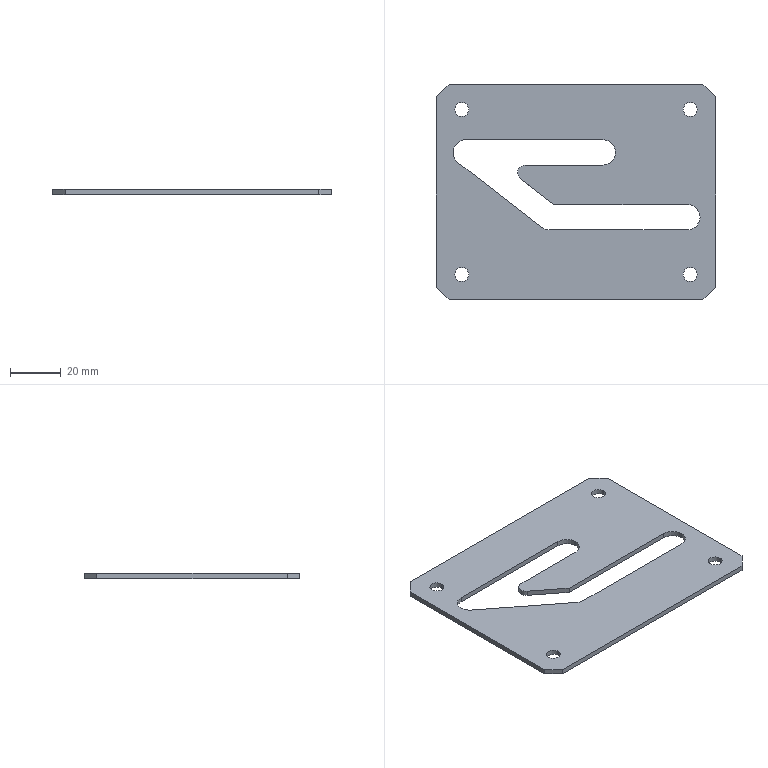Part | SolidWorks | features ICE 15, HoleWzd 5, MoveFace 2, Chamfer 1, Cut 1, Extrusion 1, Fillet 1, MirrorPattern 1 | 1 solid | 31 faces | box 110 x 85 x 2 mm | volume 15306 mm3 | plane 16 | cylinder 15 | commonest cylinder face diameters 5.5 x8 10 x6 6 x1
STEP:
#1=CARTESIAN_POINT('',(0.06,108.022,-1.));
#2=VERTEX_POINT('',#1);
#3=CARTESIAN_POINT('',(5.06,103.022,-1.));
#4=VERTEX_POINT('',#3);
#5=CARTESIAN_POINT('',(0.06,103.022,-1.));
#6=DIRECTION('',(0.,0.,-1.));
#7=DIRECTION('',(-1.,0.,0.));
#8=AXIS2_PLACEMENT_3D('',#5,#6,#7);
#9=CIRCLE('',#8,5.);
#10=EDGE_CURVE('',#2,#4,#9,.T.);
#11=ORIENTED_EDGE('',*,*,#10,.T.);
#12=CARTESIAN_POINT('',(5.06,103.022,1.));
#13=VERTEX_POINT('',#12);
#14=CARTESIAN_POINT('',(5.06,103.022,-9.));
#15=DIRECTION('',(0.,0.,1.));
#16=VECTOR('',#15,1000.);
#17=LINE('',#14,#16);
#18=EDGE_CURVE('',#4,#13,#17,.T.);
#19=ORIENTED_EDGE('',*,*,#18,.T.);
#20=CARTESIAN_POINT('',(0.06,108.022,1.));
#21=VERTEX_POINT('',#20);
#22=CARTESIAN_POINT('',(0.06,103.022,1.));
#23=DIRECTION('',(0.,0.,1.));
#24=DIRECTION('',(-1.,0.,0.));
#25=AXIS2_PLACEMENT_3D('',#22,#23,#24);
#26=CIRCLE('',#25,5.);
#27=EDGE_CURVE('',#13,#21,#26,.T.);
#28=ORIENTED_EDGE('',*,*,#27,.T.);
#29=CARTESIAN_POINT('',(0.06,108.022,-9.));
#30=DIRECTION('',(0.,0.,1.));
#31=VECTOR('',#30,1000.);
#32=LINE('',#29,#31);
#33=EDGE_CURVE('',#2,#21,#32,.T.);
#34=ORIENTED_EDGE('',*,*,#33,.F.);
#35=EDGE_LOOP('',(#11,#19,#28,#34));
#36=FACE_OUTER_BOUND('',#35,.T.);
#37=CARTESIAN_POINT('',(0.06,103.022,-9.));
#38=DIRECTION('',(0.,0.,1.));
#39=DIRECTION('',(1.,0.,0.));
#40=AXIS2_PLACEMENT_3D('',#37,#38,#39);
#41=CYLINDRICAL_SURFACE('',#40,5.);
#42=ADVANCED_FACE('',(#36),#41,.F.);
#43=CARTESIAN_POINT('',(33.36,82.489,-1.));
#44=VERTEX_POINT('',#43);
#45=CARTESIAN_POINT('',(38.36,77.489,-1.));
#46=VERTEX_POINT('',#45);
#47=CARTESIAN_POINT('',(33.36,77.489,-1.));
#48=DIRECTION('',(0.,0.,-1.));
#49=DIRECTION('',(-1.,0.,0.));
#50=AXIS2_PLACEMENT_3D('',#47,#48,#49);
#51=CIRCLE('',#50,5.);
#52=EDGE_CURVE('',#44,#46,#51,.T.);
#53=ORIENTED_EDGE('',*,*,#52,.T.);
#54=CARTESIAN_POINT('',(38.36,77.489,1.));
#55=VERTEX_POINT('',#54);
#56=CARTESIAN_POINT('',(38.36,77.489,-9.));
#57=DIRECTION('',(0.,0.,1.));
#58=VECTOR('',#57,1000.);
#59=LINE('',#56,#58);
#60=EDGE_CURVE('',#46,#55,#59,.T.);
#61=ORIENTED_EDGE('',*,*,#60,.T.);
#62=CARTESIAN_POINT('',(33.36,82.489,1.));
#63=VERTEX_POINT('',#62);
#64=CARTESIAN_POINT('',(33.36,77.489,1.));
#65=DIRECTION('',(0.,0.,1.));
#66=DIRECTION('',(-1.,0.,0.));
#67=AXIS2_PLACEMENT_3D('',#64,#65,#66);
#68=CIRCLE('',#67,5.);
#69=EDGE_CURVE('',#55,#63,#68,.T.);
#70=ORIENTED_EDGE('',*,*,#69,.T.);
#71=CARTESIAN_POINT('',(33.36,82.489,-9.));
#72=DIRECTION('',(0.,0.,1.));
#73=VECTOR('',#72,1000.);
#74=LINE('',#71,#73);
#75=EDGE_CURVE('',#44,#63,#74,.T.);
#76=ORIENTED_EDGE('',*,*,#75,.F.);
#77=EDGE_LOOP('',(#53,#61,#70,#76));
#78=FACE_OUTER_BOUND('',#77,.T.);
#79=CARTESIAN_POINT('',(33.36,77.489,-9.));
#80=DIRECTION('',(0.,0.,1.));
#81=DIRECTION('',(1.,0.,0.));
#82=AXIS2_PLACEMENT_3D('',#79,#80,#81);
#83=CYLINDRICAL_SURFACE('',#82,5.);
#84=ADVANCED_FACE('',(#78),#83,.F.);
#85=CARTESIAN_POINT('',(31.75,54.928,-1.));
#86=VERTEX_POINT('',#85);
#87=CARTESIAN_POINT('',(37.25,54.928,-1.));
#88=VERTEX_POINT('',#87);
#89=CARTESIAN_POINT('',(34.5,54.928,-1.));
#90=DIRECTION('',(0.,0.,1.));
#91=DIRECTION('',(1.,0.,0.));
#92=AXIS2_PLACEMENT_3D('',#89,#90,#91);
#93=CIRCLE('',#92,2.75);
#94=EDGE_CURVE('',#86,#88,#93,.T.);
#95=ORIENTED_EDGE('',*,*,#94,.F.);
#96=CARTESIAN_POINT('',(31.75,54.928,1.));
#97=VERTEX_POINT('',#96);
#98=CARTESIAN_POINT('',(31.75,54.928,1.));
#99=DIRECTION('',(0.,0.,1.));
#100=VECTOR('',#99,1000.);
#101=LINE('',#98,#100);
#102=EDGE_CURVE('',#86,#97,#101,.T.);
#103=ORIENTED_EDGE('',*,*,#102,.T.);
#104=CARTESIAN_POINT('',(37.25,54.928,1.));
#105=VERTEX_POINT('',#104);
#106=CARTESIAN_POINT('',(34.5,54.928,1.));
#107=DIRECTION('',(0.,0.,1.));
#108=DIRECTION('',(1.,0.,0.));
#109=AXIS2_PLACEMENT_3D('',#106,#107,#108);
#110=CIRCLE('',#109,2.75);
#111=EDGE_CURVE('',#97,#105,#110,.T.);
#112=ORIENTED_EDGE('',*,*,#111,.T.);
#113=CARTESIAN_POINT('',(37.25,54.928,1.));
#114=DIRECTION('',(0.,0.,1.));
#115=VECTOR('',#114,1000.);
#116=LINE('',#113,#115);
#117=EDGE_CURVE('',#88,#105,#116,.T.);
#118=ORIENTED_EDGE('',*,*,#117,.F.);
#119=EDGE_LOOP('',(#95,#103,#112,#118));
#120=FACE_OUTER_BOUND('',#119,.T.);
#121=CARTESIAN_POINT('',(34.5,54.928,1.));
#122=DIRECTION('',(0.,0.,1.));
#123=DIRECTION('',(1.,0.,0.));
#124=AXIS2_PLACEMENT_3D('',#121,#122,#123);
#125=CYLINDRICAL_SURFACE('',#124,2.75);
#126=ADVANCED_FACE('',(#120),#125,.F.);
#127=CARTESIAN_POINT('',(31.75,119.928,-1.));
#128=VERTEX_POINT('',#127);
#129=CARTESIAN_POINT('',(37.25,119.928,-1.));
#130=VERTEX_POINT('',#129);
#131=CARTESIAN_POINT('',(34.5,119.928,-1.));
#132=DIRECTION('',(0.,0.,1.));
#133=DIRECTION('',(1.,0.,0.));
#134=AXIS2_PLACEMENT_3D('',#131,#132,#133);
#135=CIRCLE('',#134,2.75);
#136=EDGE_CURVE('',#128,#130,#135,.T.);
#137=ORIENTED_EDGE('',*,*,#136,.F.);
#138=CARTESIAN_POINT('',(31.75,119.928,1.));
#139=VERTEX_POINT('',#138);
#140=CARTESIAN_POINT('',(31.75,119.928,1.));
#141=DIRECTION('',(0.,0.,1.));
#142=VECTOR('',#141,1000.);
#143=LINE('',#140,#142);
#144=EDGE_CURVE('',#128,#139,#143,.T.);
#145=ORIENTED_EDGE('',*,*,#144,.T.);
#146=CARTESIAN_POINT('',(37.25,119.928,1.));
#147=VERTEX_POINT('',#146);
#148=CARTESIAN_POINT('',(34.5,119.928,1.));
#149=DIRECTION('',(0.,0.,1.));
#150=DIRECTION('',(1.,0.,0.));
#151=AXIS2_PLACEMENT_3D('',#148,#149,#150);
#152=CIRCLE('',#151,2.75);
#153=EDGE_CURVE('',#139,#147,#152,.T.);
#154=ORIENTED_EDGE('',*,*,#153,.T.);
#155=CARTESIAN_POINT('',(37.25,119.928,1.));
#156=DIRECTION('',(0.,0.,1.));
#157=VECTOR('',#156,1000.);
#158=LINE('',#155,#157);
#159=EDGE_CURVE('',#130,#147,#158,.T.);
#160=ORIENTED_EDGE('',*,*,#159,.F.);
#161=EDGE_LOOP('',(#137,#145,#154,#160));
#162=FACE_OUTER_BOUND('',#161,.T.);
#163=CARTESIAN_POINT('',(34.5,119.928,1.));
#164=DIRECTION('',(0.,0.,1.));
#165=DIRECTION('',(1.,0.,0.));
#166=AXIS2_PLACEMENT_3D('',#163,#164,#165);
#167=CYLINDRICAL_SURFACE('',#166,2.75);
#168=ADVANCED_FACE('',(#162),#167,.F.);
#169=CARTESIAN_POINT('',(-58.25,119.928,-1.));
#170=VERTEX_POINT('',#169);
#171=CARTESIAN_POINT('',(-52.75,119.928,-1.));
#172=VERTEX_POINT('',#171);
#173=CARTESIAN_POINT('',(-55.5,119.928,-1.));
#174=DIRECTION('',(0.,0.,1.));
#175=DIRECTION('',(1.,0.,0.));
#176=AXIS2_PLACEMENT_3D('',#173,#174,#175);
#177=CIRCLE('',#176,2.75);
#178=EDGE_CURVE('',#170,#172,#177,.T.);
#179=ORIENTED_EDGE('',*,*,#178,.F.);
#180=CARTESIAN_POINT('',(-58.25,119.928,1.));
#181=VERTEX_POINT('',#180);
#182=CARTESIAN_POINT('',(-58.25,119.928,1.));
#183=DIRECTION('',(0.,0.,1.));
#184=VECTOR('',#183,1000.);
#185=LINE('',#182,#184);
#186=EDGE_CURVE('',#170,#181,#185,.T.);
#187=ORIENTED_EDGE('',*,*,#186,.T.);
#188=CARTESIAN_POINT('',(-52.75,119.928,1.));
#189=VERTEX_POINT('',#188);
#190=CARTESIAN_POINT('',(-55.5,119.928,1.));
#191=DIRECTION('',(0.,0.,1.));
#192=DIRECTION('',(1.,0.,0.));
#193=AXIS2_PLACEMENT_3D('',#190,#191,#192);
#194=CIRCLE('',#193,2.75);
#195=EDGE_CURVE('',#181,#189,#194,.T.);
#196=ORIENTED_EDGE('',*,*,#195,.T.);
#197=CARTESIAN_POINT('',(-52.75,119.928,1.));
#198=DIRECTION('',(0.,0.,1.));
#199=VECTOR('',#198,1000.);
#200=LINE('',#197,#199);
#201=EDGE_CURVE('',#172,#189,#200,.T.);
#202=ORIENTED_EDGE('',*,*,#201,.F.);
#203=EDGE_LOOP('',(#179,#187,#196,#202));
#204=FACE_OUTER_BOUND('',#203,.T.);
#205=CARTESIAN_POINT('',(-55.5,119.928,1.));
#206=DIRECTION('',(0.,0.,1.));
#207=DIRECTION('',(1.,0.,0.));
#208=AXIS2_PLACEMENT_3D('',#205,#206,#207);
#209=CYLINDRICAL_SURFACE('',#208,2.75);
#210=ADVANCED_FACE('',(#204),#209,.F.);
#211=CARTESIAN_POINT('',(-58.25,54.928,-1.));
#212=VERTEX_POINT('',#211);
#213=CARTESIAN_POINT('',(-52.75,54.928,-1.));
#214=VERTEX_POINT('',#213);
#215=CARTESIAN_POINT('',(-55.5,54.928,-1.));
#216=DIRECTION('',(0.,0.,1.));
#217=DIRECTION('',(1.,0.,0.));
#218=AXIS2_PLACEMENT_3D('',#215,#216,#217);
#219=CIRCLE('',#218,2.75);
#220=EDGE_CURVE('',#212,#214,#219,.T.);
#221=ORIENTED_EDGE('',*,*,#220,.F.);
#222=CARTESIAN_POINT('',(-58.25,54.928,1.));
#223=VERTEX_POINT('',#222);
#224=CARTESIAN_POINT('',(-58.25,54.928,1.));
#225=DIRECTION('',(0.,0.,1.));
#226=VECTOR('',#225,1000.);
#227=LINE('',#224,#226);
#228=EDGE_CURVE('',#212,#223,#227,.T.);
#229=ORIENTED_EDGE('',*,*,#228,.T.);
#230=CARTESIAN_POINT('',(-52.75,54.928,1.));
#231=VERTEX_POINT('',#230);
#232=CARTESIAN_POINT('',(-55.5,54.928,1.));
#233=DIRECTION('',(0.,0.,1.));
#234=DIRECTION('',(1.,0.,0.));
#235=AXIS2_PLACEMENT_3D('',#232,#233,#234);
#236=CIRCLE('',#235,2.75);
#237=EDGE_CURVE('',#223,#231,#236,.T.);
#238=ORIENTED_EDGE('',*,*,#237,.T.);
#239=CARTESIAN_POINT('',(-52.75,54.928,1.));
#240=DIRECTION('',(0.,0.,1.));
#241=VECTOR('',#240,1000.);
#242=LINE('',#239,#241);
#243=EDGE_CURVE('',#214,#231,#242,.T.);
#244=ORIENTED_EDGE('',*,*,#243,.F.);
#245=EDGE_LOOP('',(#221,#229,#238,#244));
#246=FACE_OUTER_BOUND('',#245,.T.);
#247=CARTESIAN_POINT('',(-55.5,54.928,1.));
#248=DIRECTION('',(0.,0.,1.));
#249=DIRECTION('',(1.,0.,0.));
#250=AXIS2_PLACEMENT_3D('',#247,#248,#249);
#251=CYLINDRICAL_SURFACE('',#250,2.75);
#252=ADVANCED_FACE('',(#246),#251,.F.);
#253=CARTESIAN_POINT('',(-19.302,82.489,1.));
#254=VERTEX_POINT('',#253);
#255=CARTESIAN_POINT('',(33.36,82.489,1.));
#256=DIRECTION('',(-1.,0.,0.));
#257=VECTOR('',#256,1000.);
#258=LINE('',#255,#257);
#259=EDGE_CURVE('',#63,#254,#258,.T.);
#260=ORIENTED_EDGE('',*,*,#259,.F.);
#261=ORIENTED_EDGE('',*,*,#69,.F.);
#262=CARTESIAN_POINT('',(33.36,72.489,1.));
#263=VERTEX_POINT('',#262);
#264=CARTESIAN_POINT('',(33.36,77.489,1.));
#265=DIRECTION('',(0.,0.,1.));
#266=DIRECTION('',(-1.,0.,0.));
#267=AXIS2_PLACEMENT_3D('',#264,#265,#266);
#268=CIRCLE('',#267,5.);
#269=EDGE_CURVE('',#263,#55,#268,.T.);
#270=ORIENTED_EDGE('',*,*,#269,.F.);
#271=CARTESIAN_POINT('',(-21.013,72.489,1.));
#272=VERTEX_POINT('',#271);
#273=CARTESIAN_POINT('',(33.36,72.489,1.));
#274=DIRECTION('',(1.,0.,0.));
#275=VECTOR('',#274,1000.);
#276=LINE('',#273,#275);
#277=EDGE_CURVE('',#272,#263,#276,.T.);
#278=ORIENTED_EDGE('',*,*,#277,.F.);
#279=CARTESIAN_POINT('',(-24.076,73.537,1.));
#280=VERTEX_POINT('',#279);
#281=CARTESIAN_POINT('',(-21.013,77.489,1.));
#282=DIRECTION('',(0.,0.,1.));
#283=DIRECTION('',(-1.,0.,0.));
#284=AXIS2_PLACEMENT_3D('',#281,#282,#283);
#285=CIRCLE('',#284,5.);
#286=EDGE_CURVE('',#280,#272,#285,.T.);
#287=ORIENTED_EDGE('',*,*,#286,.F.);
#288=CARTESIAN_POINT('',(-57.018,99.07,1.));
#289=VERTEX_POINT('',#288);
#290=CARTESIAN_POINT('',(-24.076,73.537,1.));
#291=DIRECTION('',(0.7904,-0.6126,0.));
#292=VECTOR('',#291,1000.);
#293=LINE('',#290,#292);
#294=EDGE_CURVE('',#289,#280,#293,.T.);
#295=ORIENTED_EDGE('',*,*,#294,.F.);
#296=CARTESIAN_POINT('',(-53.955,108.022,1.));
#297=VERTEX_POINT('',#296);
#298=CARTESIAN_POINT('',(-53.955,103.022,1.));
#299=DIRECTION('',(0.,0.,1.));
#300=DIRECTION('',(1.,0.,0.));
#301=AXIS2_PLACEMENT_3D('',#298,#299,#300);
#302=CIRCLE('',#301,5.);
#303=EDGE_CURVE('',#297,#289,#302,.T.);
#304=ORIENTED_EDGE('',*,*,#303,.F.);
#305=CARTESIAN_POINT('',(0.06,108.022,1.));
#306=DIRECTION('',(-1.,0.,0.));
#307=VECTOR('',#306,1000.);
#308=LINE('',#305,#307);
#309=EDGE_CURVE('',#21,#297,#308,.T.);
#310=ORIENTED_EDGE('',*,*,#309,.F.);
#311=ORIENTED_EDGE('',*,*,#27,.F.);
#312=CARTESIAN_POINT('',(0.06,98.022,1.));
#313=VERTEX_POINT('',#312);
#314=CARTESIAN_POINT('',(0.06,103.022,1.));
#315=DIRECTION('',(0.,0.,1.));
#316=DIRECTION('',(-1.,0.,0.));
#317=AXIS2_PLACEMENT_3D('',#314,#315,#316);
#318=CIRCLE('',#317,5.);
#319=EDGE_CURVE('',#313,#13,#318,.T.);
#320=ORIENTED_EDGE('',*,*,#319,.F.);
#321=CARTESIAN_POINT('',(-30.575,98.022,1.));
#322=VERTEX_POINT('',#321);
#323=CARTESIAN_POINT('',(0.06,98.022,1.));
#324=DIRECTION('',(1.,0.,0.));
#325=VECTOR('',#324,1000.);
#326=LINE('',#323,#325);
#327=EDGE_CURVE('',#322,#313,#326,.T.);
#328=ORIENTED_EDGE('',*,*,#327,.F.);
#329=CARTESIAN_POINT('',(-32.412,92.65,1.));
#330=VERTEX_POINT('',#329);
#331=CARTESIAN_POINT('',(-30.575,95.022,1.));
#332=DIRECTION('',(0.,0.,-1.));
#333=DIRECTION('',(1.,0.,0.));
#334=AXIS2_PLACEMENT_3D('',#331,#332,#333);
#335=CIRCLE('',#334,3.);
#336=EDGE_CURVE('',#330,#322,#335,.T.);
#337=ORIENTED_EDGE('',*,*,#336,.F.);
#338=CARTESIAN_POINT('',(-19.302,82.489,1.));
#339=DIRECTION('',(-0.7904,0.6126,0.));
#340=VECTOR('',#339,1000.);
#341=LINE('',#338,#340);
#342=EDGE_CURVE('',#254,#330,#341,.T.);
#343=ORIENTED_EDGE('',*,*,#342,.F.);
#344=EDGE_LOOP('',(#260,#261,#270,#278,#287,#295,#304,#310,#311,#320,#328,#337,#343));
#345=FACE_BOUND('',#344,.T.);
#346=CARTESIAN_POINT('',(34.5,54.928,1.));
#347=DIRECTION('',(0.,0.,1.));
#348=DIRECTION('',(1.,0.,0.));
#349=AXIS2_PLACEMENT_3D('',#346,#347,#348);
#350=CIRCLE('',#349,2.75);
#351=EDGE_CURVE('',#105,#97,#350,.T.);
#352=ORIENTED_EDGE('',*,*,#351,.F.);
#353=ORIENTED_EDGE('',*,*,#111,.F.);
#354=EDGE_LOOP('',(#352,#353));
#355=FACE_BOUND('',#354,.T.);
#356=CARTESIAN_POINT('',(34.5,119.928,1.));
#357=DIRECTION('',(0.,0.,1.));
#358=DIRECTION('',(1.,0.,0.));
#359=AXIS2_PLACEMENT_3D('',#356,#357,#358);
#360=CIRCLE('',#359,2.75);
#361=EDGE_CURVE('',#147,#139,#360,.T.);
#362=ORIENTED_EDGE('',*,*,#361,.F.);
#363=ORIENTED_EDGE('',*,*,#153,.F.);
#364=EDGE_LOOP('',(#362,#363));
#365=FACE_BOUND('',#364,.T.);
#366=CARTESIAN_POINT('',(-55.5,119.928,1.));
#367=DIRECTION('',(0.,0.,1.));
#368=DIRECTION('',(1.,0.,0.));
#369=AXIS2_PLACEMENT_3D('',#366,#367,#368);
#370=CIRCLE('',#369,2.75);
#371=EDGE_CURVE('',#189,#181,#370,.T.);
#372=ORIENTED_EDGE('',*,*,#371,.F.);
#373=ORIENTED_EDGE('',*,*,#195,.F.);
#374=EDGE_LOOP('',(#372,#373));
#375=FACE_BOUND('',#374,.T.);
#376=CARTESIAN_POINT('',(-55.5,54.928,1.));
#377=DIRECTION('',(0.,0.,1.));
#378=DIRECTION('',(1.,0.,0.));
#379=AXIS2_PLACEMENT_3D('',#376,#377,#378);
#380=CIRCLE('',#379,2.75);
#381=EDGE_CURVE('',#231,#223,#380,.T.);
#382=ORIENTED_EDGE('',*,*,#381,.F.);
#383=ORIENTED_EDGE('',*,*,#237,.F.);
#384=EDGE_LOOP('',(#382,#383));
#385=FACE_BOUND('',#384,.T.);
#386=CARTESIAN_POINT('',(39.5,129.928,1.));
#387=VERTEX_POINT('',#386);
#388=CARTESIAN_POINT('',(-60.5,129.928,1.));
#389=VERTEX_POINT('',#388);
#390=CARTESIAN_POINT('',(-65.5,129.928,1.));
#391=DIRECTION('',(-1.,0.,0.));
#392=VECTOR('',#391,1000.);
#393=LINE('',#390,#392);
#394=EDGE_CURVE('',#387,#389,#393,.T.);
#395=ORIENTED_EDGE('',*,*,#394,.T.);
#396=CARTESIAN_POINT('',(-65.5,124.928,1.));
#397=VERTEX_POINT('',#396);
#398=CARTESIAN_POINT('',(-60.5,129.928,1.));
#399=DIRECTION('',(-0.7071,-0.7071,0.));
#400=VECTOR('',#399,1000.);
#401=LINE('',#398,#400);
#402=EDGE_CURVE('',#389,#397,#401,.T.);
#403=ORIENTED_EDGE('',*,*,#402,.T.);
#404=CARTESIAN_POINT('',(-65.5,49.928,1.));
#405=VERTEX_POINT('',#404);
#406=CARTESIAN_POINT('',(-65.5,129.928,1.));
#407=DIRECTION('',(0.,-1.,0.));
#408=VECTOR('',#407,1000.);
#409=LINE('',#406,#408);
#410=EDGE_CURVE('',#397,#405,#409,.T.);
#411=ORIENTED_EDGE('',*,*,#410,.T.);
#412=CARTESIAN_POINT('',(-60.5,44.928,1.));
#413=VERTEX_POINT('',#412);
#414=CARTESIAN_POINT('',(-65.5,49.928,1.));
#415=DIRECTION('',(0.7071,-0.7071,0.));
#416=VECTOR('',#415,1000.);
#417=LINE('',#414,#416);
#418=EDGE_CURVE('',#405,#413,#417,.T.);
#419=ORIENTED_EDGE('',*,*,#418,.T.);
#420=CARTESIAN_POINT('',(39.5,44.928,1.));
#421=VERTEX_POINT('',#420);
#422=CARTESIAN_POINT('',(-65.5,44.928,1.));
#423=DIRECTION('',(1.,0.,0.));
#424=VECTOR('',#423,1000.);
#425=LINE('',#422,#424);
#426=EDGE_CURVE('',#413,#421,#425,.T.);
#427=ORIENTED_EDGE('',*,*,#426,.T.);
#428=CARTESIAN_POINT('',(44.5,49.928,1.));
#429=VERTEX_POINT('',#428);
#430=CARTESIAN_POINT('',(39.5,44.928,1.));
#431=DIRECTION('',(0.7071,0.7071,0.));
#432=VECTOR('',#431,1000.);
#433=LINE('',#430,#432);
#434=EDGE_CURVE('',#421,#429,#433,.T.);
#435=ORIENTED_EDGE('',*,*,#434,.T.);
#436=CARTESIAN_POINT('',(44.5,124.928,1.));
#437=VERTEX_POINT('',#436);
#438=CARTESIAN_POINT('',(44.5,129.928,1.));
#439=DIRECTION('',(0.,1.,0.));
#440=VECTOR('',#439,1000.);
#441=LINE('',#438,#440);
#442=EDGE_CURVE('',#429,#437,#441,.T.);
#443=ORIENTED_EDGE('',*,*,#442,.T.);
#444=CARTESIAN_POINT('',(44.5,124.928,1.));
#445=DIRECTION('',(-0.7071,0.7071,0.));
#446=VECTOR('',#445,1000.);
#447=LINE('',#444,#446);
#448=EDGE_CURVE('',#437,#387,#447,.T.);
#449=ORIENTED_EDGE('',*,*,#448,.T.);
#450=EDGE_LOOP('',(#395,#403,#411,#419,#427,#435,#443,#449));
#451=FACE_OUTER_BOUND('',#450,.T.);
#452=CARTESIAN_POINT('',(66.5,86.298,1.));
#453=DIRECTION('',(0.,0.,-1.));
#454=DIRECTION('',(-1.,0.,0.));
#455=AXIS2_PLACEMENT_3D('',#452,#453,#454);
#456=PLANE('',#455);
#457=ADVANCED_FACE('',(#345,#355,#365,#375,#385,#451),#456,.F.);
#458=ORIENTED_EDGE('',*,*,#410,.F.);
#459=CARTESIAN_POINT('',(-65.5,124.928,-1.));
#460=VERTEX_POINT('',#459);
#461=CARTESIAN_POINT('',(-65.5,124.928,-1.));
#462=DIRECTION('',(0.,0.,-1.));
#463=VECTOR('',#462,1000.);
#464=LINE('',#461,#463);
#465=EDGE_CURVE('',#397,#460,#464,.T.);
#466=ORIENTED_EDGE('',*,*,#465,.T.);
#467=CARTESIAN_POINT('',(-65.5,49.928,-1.));
#468=VERTEX_POINT('',#467);
#469=CARTESIAN_POINT('',(-65.5,129.928,-1.));
#470=DIRECTION('',(0.,-1.,0.));
#471=VECTOR('',#470,1000.);
#472=LINE('',#469,#471);
#473=EDGE_CURVE('',#460,#468,#472,.T.);
#474=ORIENTED_EDGE('',*,*,#473,.T.);
#475=CARTESIAN_POINT('',(-65.5,49.928,-1.));
#476=DIRECTION('',(0.,0.,1.));
#477=VECTOR('',#476,1000.);
#478=LINE('',#475,#477);
#479=EDGE_CURVE('',#468,#405,#478,.T.);
#480=ORIENTED_EDGE('',*,*,#479,.T.);
#481=EDGE_LOOP('',(#458,#466,#474,#480));
#482=FACE_OUTER_BOUND('',#481,.T.);
#483=CARTESIAN_POINT('',(-65.5,129.928,-1.));
#484=DIRECTION('',(-1.,0.,0.));
#485=DIRECTION('',(0.,0.,1.));
#486=AXIS2_PLACEMENT_3D('',#483,#484,#485);
#487=PLANE('',#486);
#488=ADVANCED_FACE('',(#482),#487,.T.);
#489=CARTESIAN_POINT('',(39.5,129.928,-1.));
#490=VERTEX_POINT('',#489);
#491=CARTESIAN_POINT('',(-60.5,129.928,-1.));
#492=VERTEX_POINT('',#491);
#493=CARTESIAN_POINT('',(-65.5,129.928,-1.));
#494=DIRECTION('',(-1.,0.,0.));
#495=VECTOR('',#494,1000.);
#496=LINE('',#493,#495);
#497=EDGE_CURVE('',#490,#492,#496,.T.);
#498=ORIENTED_EDGE('',*,*,#497,.T.);
#499=CARTESIAN_POINT('',(-60.5,129.928,-1.));
#500=DIRECTION('',(0.,0.,1.));
#501=VECTOR('',#500,1000.);
#502=LINE('',#499,#501);
#503=EDGE_CURVE('',#492,#389,#502,.T.);
#504=ORIENTED_EDGE('',*,*,#503,.T.);
#505=ORIENTED_EDGE('',*,*,#394,.F.);
#506=CARTESIAN_POINT('',(39.5,129.928,-1.));
#507=DIRECTION('',(0.,0.,-1.));
#508=VECTOR('',#507,1000.);
#509=LINE('',#506,#508);
#510=EDGE_CURVE('',#387,#490,#509,.T.);
#511=ORIENTED_EDGE('',*,*,#510,.T.);
#512=EDGE_LOOP('',(#498,#504,#505,#511));
#513=FACE_OUTER_BOUND('',#512,.T.);
#514=CARTESIAN_POINT('',(-65.5,129.928,-1.));
#515=DIRECTION('',(0.,1.,0.));
#516=DIRECTION('',(0.,0.,1.));
#517=AXIS2_PLACEMENT_3D('',#514,#515,#516);
#518=PLANE('',#517);
#519=ADVANCED_FACE('',(#513),#518,.T.);
#520=CARTESIAN_POINT('',(44.5,49.928,-1.));
#521=VERTEX_POINT('',#520);
#522=CARTESIAN_POINT('',(44.5,124.928,-1.));
#523=VERTEX_POINT('',#522);
#524=CARTESIAN_POINT('',(44.5,129.928,-1.));
#525=DIRECTION('',(0.,1.,0.));
#526=VECTOR('',#525,1000.);
#527=LINE('',#524,#526);
#528=EDGE_CURVE('',#521,#523,#527,.T.);
#529=ORIENTED_EDGE('',*,*,#528,.T.);
#530=CARTESIAN_POINT('',(44.5,124.928,-1.));
#531=DIRECTION('',(0.,0.,1.));
#532=VECTOR('',#531,1000.);
#533=LINE('',#530,#532);
#534=EDGE_CURVE('',#523,#437,#533,.T.);
#535=ORIENTED_EDGE('',*,*,#534,.T.);
#536=ORIENTED_EDGE('',*,*,#442,.F.);
#537=CARTESIAN_POINT('',(44.5,49.928,-1.));
#538=DIRECTION('',(0.,0.,-1.));
#539=VECTOR('',#538,1000.);
#540=LINE('',#537,#539);
#541=EDGE_CURVE('',#429,#521,#540,.T.);
#542=ORIENTED_EDGE('',*,*,#541,.T.);
#543=EDGE_LOOP('',(#529,#535,#536,#542));
#544=FACE_OUTER_BOUND('',#543,.T.);
#545=CARTESIAN_POINT('',(44.5,129.928,-1.));
#546=DIRECTION('',(1.,0.,0.));
#547=DIRECTION('',(0.,1.,0.));
#548=AXIS2_PLACEMENT_3D('',#545,#546,#547);
#549=PLANE('',#548);
#550=ADVANCED_FACE('',(#544),#549,.T.);
#551=CARTESIAN_POINT('',(-60.5,44.928,-1.));
#552=VERTEX_POINT('',#551);
#553=CARTESIAN_POINT('',(39.5,44.928,-1.));
#554=VERTEX_POINT('',#553);
#555=CARTESIAN_POINT('',(-65.5,44.928,-1.));
#556=DIRECTION('',(1.,0.,0.));
#557=VECTOR('',#556,1000.);
#558=LINE('',#555,#557);
#559=EDGE_CURVE('',#552,#554,#558,.T.);
#560=ORIENTED_EDGE('',*,*,#559,.T.);
#561=CARTESIAN_POINT('',(39.5,44.928,-1.));
#562=DIRECTION('',(0.,0.,1.));
#563=VECTOR('',#562,1000.);
#564=LINE('',#561,#563);
#565=EDGE_CURVE('',#554,#421,#564,.T.);
#566=ORIENTED_EDGE('',*,*,#565,.T.);
#567=ORIENTED_EDGE('',*,*,#426,.F.);
#568=CARTESIAN_POINT('',(-60.5,44.928,-1.));
#569=DIRECTION('',(0.,0.,-1.));
#570=VECTOR('',#569,1000.);
#571=LINE('',#568,#570);
#572=EDGE_CURVE('',#413,#552,#571,.T.);
#573=ORIENTED_EDGE('',*,*,#572,.T.);
#574=EDGE_LOOP('',(#560,#566,#567,#573));
#575=FACE_OUTER_BOUND('',#574,.T.);
#576=CARTESIAN_POINT('',(-65.5,44.928,-1.));
#577=DIRECTION('',(0.,-1.,0.));
#578=DIRECTION('',(0.,0.,-1.));
#579=AXIS2_PLACEMENT_3D('',#576,#577,#578);
#580=PLANE('',#579);
#581=ADVANCED_FACE('',(#575),#580,.T.);
#582=ORIENTED_EDGE('',*,*,#52,.F.);
#583=CARTESIAN_POINT('',(-19.302,82.489,-1.));
#584=VERTEX_POINT('',#583);
#585=CARTESIAN_POINT('',(66.5,82.489,-1.));
#586=DIRECTION('',(1.,0.,0.));
#587=VECTOR('',#586,1000.);
#588=LINE('',#585,#587);
#589=EDGE_CURVE('',#584,#44,#588,.T.);
#590=ORIENTED_EDGE('',*,*,#589,.F.);
#591=CARTESIAN_POINT('',(-32.412,92.65,-1.));
#592=VERTEX_POINT('',#591);
#593=CARTESIAN_POINT('',(32.455,42.373,-1.));
#594=DIRECTION('',(0.7904,-0.6126,0.));
#595=VECTOR('',#594,1000.);
#596=LINE('',#593,#595);
#597=EDGE_CURVE('',#592,#584,#596,.T.);
#598=ORIENTED_EDGE('',*,*,#597,.F.);
#599=CARTESIAN_POINT('',(-30.575,98.022,-1.));
#600=VERTEX_POINT('',#599);
#601=CARTESIAN_POINT('',(-30.575,95.022,-1.));
#602=DIRECTION('',(0.,0.,1.));
#603=DIRECTION('',(-1.,0.,0.));
#604=AXIS2_PLACEMENT_3D('',#601,#602,#603);
#605=CIRCLE('',#604,3.);
#606=EDGE_CURVE('',#600,#592,#605,.T.);
#607=ORIENTED_EDGE('',*,*,#606,.F.);
#608=CARTESIAN_POINT('',(0.06,98.022,-1.));
#609=VERTEX_POINT('',#608);
#610=CARTESIAN_POINT('',(66.5,98.022,-1.));
#611=DIRECTION('',(-1.,0.,0.));
#612=VECTOR('',#611,1000.);
#613=LINE('',#610,#612);
#614=EDGE_CURVE('',#609,#600,#613,.T.);
#615=ORIENTED_EDGE('',*,*,#614,.F.);
#616=CARTESIAN_POINT('',(0.06,103.022,-1.));
#617=DIRECTION('',(0.,0.,-1.));
#618=DIRECTION('',(-1.,0.,0.));
#619=AXIS2_PLACEMENT_3D('',#616,#617,#618);
#620=CIRCLE('',#619,5.);
#621=EDGE_CURVE('',#4,#609,#620,.T.);
#622=ORIENTED_EDGE('',*,*,#621,.F.);
#623=ORIENTED_EDGE('',*,*,#10,.F.);
#624=CARTESIAN_POINT('',(-53.955,108.022,-1.));
#625=VERTEX_POINT('',#624);
#626=CARTESIAN_POINT('',(66.5,108.022,-1.));
#627=DIRECTION('',(1.,0.,0.));
#628=VECTOR('',#627,1000.);
#629=LINE('',#626,#628);
#630=EDGE_CURVE('',#625,#2,#629,.T.);
#631=ORIENTED_EDGE('',*,*,#630,.F.);
#632=CARTESIAN_POINT('',(-57.018,99.07,-1.));
#633=VERTEX_POINT('',#632);
#634=CARTESIAN_POINT('',(-53.955,103.022,-1.));
#635=DIRECTION('',(0.,0.,-1.));
#636=DIRECTION('',(-1.,0.,0.));
#637=AXIS2_PLACEMENT_3D('',#634,#635,#636);
#638=CIRCLE('',#637,5.);
#639=EDGE_CURVE('',#633,#625,#638,.T.);
#640=ORIENTED_EDGE('',*,*,#639,.F.);
#641=CARTESIAN_POINT('',(-24.076,73.537,-1.));
#642=VERTEX_POINT('',#641);
#643=CARTESIAN_POINT('',(26.329,34.469,-1.));
#644=DIRECTION('',(-0.7904,0.6126,0.));
#645=VECTOR('',#644,1000.);
#646=LINE('',#643,#645);
#647=EDGE_CURVE('',#642,#633,#646,.T.);
#648=ORIENTED_EDGE('',*,*,#647,.F.);
#649=CARTESIAN_POINT('',(-21.013,72.489,-1.));
#650=VERTEX_POINT('',#649);
#651=CARTESIAN_POINT('',(-21.013,77.489,-1.));
#652=DIRECTION('',(0.,0.,-1.));
#653=DIRECTION('',(-1.,0.,0.));
#654=AXIS2_PLACEMENT_3D('',#651,#652,#653);
#655=CIRCLE('',#654,5.);
#656=EDGE_CURVE('',#650,#642,#655,.T.);
#657=ORIENTED_EDGE('',*,*,#656,.F.);
#658=CARTESIAN_POINT('',(33.36,72.489,-1.));
#659=VERTEX_POINT('',#658);
#660=CARTESIAN_POINT('',(66.5,72.489,-1.));
#661=DIRECTION('',(-1.,0.,0.));
#662=VECTOR('',#661,1000.);
#663=LINE('',#660,#662);
#664=EDGE_CURVE('',#659,#650,#663,.T.);
#665=ORIENTED_EDGE('',*,*,#664,.F.);
#666=CARTESIAN_POINT('',(33.36,77.489,-1.));
#667=DIRECTION('',(0.,0.,-1.));
#668=DIRECTION('',(-1.,0.,0.));
#669=AXIS2_PLACEMENT_3D('',#666,#667,#668);
#670=CIRCLE('',#669,5.);
#671=EDGE_CURVE('',#46,#659,#670,.T.);
#672=ORIENTED_EDGE('',*,*,#671,.F.);
#673=EDGE_LOOP('',(#582,#590,#598,#607,#615,#622,#623,#631,#640,#648,#657,#665,#672));
#674=FACE_BOUND('',#673,.T.);
#675=CARTESIAN_POINT('',(34.5,54.928,-1.));
#676=DIRECTION('',(0.,0.,1.));
#677=DIRECTION('',(1.,0.,0.));
#678=AXIS2_PLACEMENT_3D('',#675,#676,#677);
#679=CIRCLE('',#678,2.75);
#680=EDGE_CURVE('',#88,#86,#679,.T.);
#681=ORIENTED_EDGE('',*,*,#680,.T.);
#682=ORIENTED_EDGE('',*,*,#94,.T.);
#683=EDGE_LOOP('',(#681,#682));
#684=FACE_BOUND('',#683,.T.);
#685=CARTESIAN_POINT('',(34.5,119.928,-1.));
#686=DIRECTION('',(0.,0.,1.));
#687=DIRECTION('',(1.,0.,0.));
#688=AXIS2_PLACEMENT_3D('',#685,#686,#687);
#689=CIRCLE('',#688,2.75);
#690=EDGE_CURVE('',#130,#128,#689,.T.);
#691=ORIENTED_EDGE('',*,*,#690,.T.);
#692=ORIENTED_EDGE('',*,*,#136,.T.);
#693=EDGE_LOOP('',(#691,#692));
#694=FACE_BOUND('',#693,.T.);
#695=CARTESIAN_POINT('',(-55.5,119.928,-1.));
#696=DIRECTION('',(0.,0.,1.));
#697=DIRECTION('',(1.,0.,0.));
#698=AXIS2_PLACEMENT_3D('',#695,#696,#697);
#699=CIRCLE('',#698,2.75);
#700=EDGE_CURVE('',#172,#170,#699,.T.);
#701=ORIENTED_EDGE('',*,*,#700,.T.);
#702=ORIENTED_EDGE('',*,*,#178,.T.);
#703=EDGE_LOOP('',(#701,#702));
#704=FACE_BOUND('',#703,.T.);
#705=CARTESIAN_POINT('',(-55.5,54.928,-1.));
#706=DIRECTION('',(0.,0.,1.));
#707=DIRECTION('',(1.,0.,0.));
#708=AXIS2_PLACEMENT_3D('',#705,#706,#707);
#709=CIRCLE('',#708,2.75);
#710=EDGE_CURVE('',#214,#212,#709,.T.);
#711=ORIENTED_EDGE('',*,*,#710,.T.);
#712=ORIENTED_EDGE('',*,*,#220,.T.);
#713=EDGE_LOOP('',(#711,#712));
#714=FACE_BOUND('',#713,.T.);
#715=ORIENTED_EDGE('',*,*,#473,.F.);
#716=CARTESIAN_POINT('',(-18.815,171.613,-1.));
#717=DIRECTION('',(0.7071,0.7071,0.));
#718=VECTOR('',#717,1000.);
#719=LINE('',#716,#718);
#720=EDGE_CURVE('',#460,#492,#719,.T.);
#721=ORIENTED_EDGE('',*,*,#720,.T.);
#722=ORIENTED_EDGE('',*,*,#497,.F.);
#723=CARTESIAN_POINT('',(74.815,94.613,-1.));
#724=DIRECTION('',(0.7071,-0.7071,0.));
#725=VECTOR('',#724,1000.);
#726=LINE('',#723,#725);
#727=EDGE_CURVE('',#490,#523,#726,.T.);
#728=ORIENTED_EDGE('',*,*,#727,.T.);
#729=ORIENTED_EDGE('',*,*,#528,.F.);
#730=CARTESIAN_POINT('',(73.685,79.113,-1.));
#731=DIRECTION('',(-0.7071,-0.7071,0.));
#732=VECTOR('',#731,1000.);
#733=LINE('',#730,#732);
#734=EDGE_CURVE('',#521,#554,#733,.T.);
#735=ORIENTED_EDGE('',*,*,#734,.T.);
#736=ORIENTED_EDGE('',*,*,#559,.F.);
#737=CARTESIAN_POINT('',(-17.685,2.113,-1.));
#738=DIRECTION('',(-0.7071,0.7071,0.));
#739=VECTOR('',#738,1000.);
#740=LINE('',#737,#739);
#741=EDGE_CURVE('',#552,#468,#740,.T.);
#742=ORIENTED_EDGE('',*,*,#741,.T.);
#743=EDGE_LOOP('',(#715,#721,#722,#728,#729,#735,#736,#742));
#744=FACE_OUTER_BOUND('',#743,.T.);
#745=CARTESIAN_POINT('',(66.5,86.298,-1.));
#746=DIRECTION('',(0.,0.,-1.));
#747=DIRECTION('',(-1.,0.,0.));
#748=AXIS2_PLACEMENT_3D('',#745,#746,#747);
#749=PLANE('',#748);
#750=ADVANCED_FACE('',(#674,#684,#694,#704,#714,#744),#749,.T.);
#751=ORIENTED_EDGE('',*,*,#720,.F.);
#752=ORIENTED_EDGE('',*,*,#465,.F.);
#753=ORIENTED_EDGE('',*,*,#402,.F.);
#754=ORIENTED_EDGE('',*,*,#503,.F.);
#755=EDGE_LOOP('',(#751,#752,#753,#754));
#756=FACE_OUTER_BOUND('',#755,.T.);
#757=CARTESIAN_POINT('',(-60.5,129.928,-1.));
#758=DIRECTION('',(0.7071,-0.7071,0.));
#759=DIRECTION('',(0.,0.,1.));
#760=AXIS2_PLACEMENT_3D('',#757,#758,#759);
#761=PLANE('',#760);
#762=ADVANCED_FACE('',(#756),#761,.F.);
#763=ORIENTED_EDGE('',*,*,#727,.F.);
#764=ORIENTED_EDGE('',*,*,#510,.F.);
#765=ORIENTED_EDGE('',*,*,#448,.F.);
#766=ORIENTED_EDGE('',*,*,#534,.F.);
#767=EDGE_LOOP('',(#763,#764,#765,#766));
#768=FACE_OUTER_BOUND('',#767,.T.);
#769=CARTESIAN_POINT('',(44.5,124.928,-1.));
#770=DIRECTION('',(-0.7071,-0.7071,0.));
#771=DIRECTION('',(0.,0.,1.));
#772=AXIS2_PLACEMENT_3D('',#769,#770,#771);
#773=PLANE('',#772);
#774=ADVANCED_FACE('',(#768),#773,.F.);
#775=ORIENTED_EDGE('',*,*,#734,.F.);
#776=ORIENTED_EDGE('',*,*,#541,.F.);
#777=ORIENTED_EDGE('',*,*,#434,.F.);
#778=ORIENTED_EDGE('',*,*,#565,.F.);
#779=EDGE_LOOP('',(#775,#776,#777,#778));
#780=FACE_OUTER_BOUND('',#779,.T.);
#781=CARTESIAN_POINT('',(39.5,44.928,-1.));
#782=DIRECTION('',(-0.7071,0.7071,0.));
#783=DIRECTION('',(0.,0.,1.));
#784=AXIS2_PLACEMENT_3D('',#781,#782,#783);
#785=PLANE('',#784);
#786=ADVANCED_FACE('',(#780),#785,.F.);
#787=ORIENTED_EDGE('',*,*,#741,.F.);
#788=ORIENTED_EDGE('',*,*,#572,.F.);
#789=ORIENTED_EDGE('',*,*,#418,.F.);
#790=ORIENTED_EDGE('',*,*,#479,.F.);
#791=EDGE_LOOP('',(#787,#788,#789,#790));
#792=FACE_OUTER_BOUND('',#791,.T.);
#793=CARTESIAN_POINT('',(-65.5,49.928,-1.));
#794=DIRECTION('',(0.7071,0.7071,0.));
#795=DIRECTION('',(0.,0.,1.));
#796=AXIS2_PLACEMENT_3D('',#793,#794,#795);
#797=PLANE('',#796);
#798=ADVANCED_FACE('',(#792),#797,.F.);
#799=ORIENTED_EDGE('',*,*,#228,.F.);
#800=ORIENTED_EDGE('',*,*,#710,.F.);
#801=ORIENTED_EDGE('',*,*,#243,.T.);
#802=ORIENTED_EDGE('',*,*,#381,.T.);
#803=EDGE_LOOP('',(#799,#800,#801,#802));
#804=FACE_OUTER_BOUND('',#803,.T.);
#805=CARTESIAN_POINT('',(-55.5,54.928,1.));
#806=DIRECTION('',(0.,0.,1.));
#807=DIRECTION('',(1.,0.,0.));
#808=AXIS2_PLACEMENT_3D('',#805,#806,#807);
#809=CYLINDRICAL_SURFACE('',#808,2.75);
#810=ADVANCED_FACE('',(#804),#809,.F.);
#811=ORIENTED_EDGE('',*,*,#186,.F.);
#812=ORIENTED_EDGE('',*,*,#700,.F.);
#813=ORIENTED_EDGE('',*,*,#201,.T.);
#814=ORIENTED_EDGE('',*,*,#371,.T.);
#815=EDGE_LOOP('',(#811,#812,#813,#814));
#816=FACE_OUTER_BOUND('',#815,.T.);
#817=CARTESIAN_POINT('',(-55.5,119.928,1.));
#818=DIRECTION('',(0.,0.,1.));
#819=DIRECTION('',(1.,0.,0.));
#820=AXIS2_PLACEMENT_3D('',#817,#818,#819);
#821=CYLINDRICAL_SURFACE('',#820,2.75);
#822=ADVANCED_FACE('',(#816),#821,.F.);
#823=ORIENTED_EDGE('',*,*,#144,.F.);
#824=ORIENTED_EDGE('',*,*,#690,.F.);
#825=ORIENTED_EDGE('',*,*,#159,.T.);
#826=ORIENTED_EDGE('',*,*,#361,.T.);
#827=EDGE_LOOP('',(#823,#824,#825,#826));
#828=FACE_OUTER_BOUND('',#827,.T.);
#829=CARTESIAN_POINT('',(34.5,119.928,1.));
#830=DIRECTION('',(0.,0.,1.));
#831=DIRECTION('',(1.,0.,0.));
#832=AXIS2_PLACEMENT_3D('',#829,#830,#831);
#833=CYLINDRICAL_SURFACE('',#832,2.75);
#834=ADVANCED_FACE('',(#828),#833,.F.);
#835=ORIENTED_EDGE('',*,*,#102,.F.);
#836=ORIENTED_EDGE('',*,*,#680,.F.);
#837=ORIENTED_EDGE('',*,*,#117,.T.);
#838=ORIENTED_EDGE('',*,*,#351,.T.);
#839=EDGE_LOOP('',(#835,#836,#837,#838));
#840=FACE_OUTER_BOUND('',#839,.T.);
#841=CARTESIAN_POINT('',(34.5,54.928,1.));
#842=DIRECTION('',(0.,0.,1.));
#843=DIRECTION('',(1.,0.,0.));
#844=AXIS2_PLACEMENT_3D('',#841,#842,#843);
#845=CYLINDRICAL_SURFACE('',#844,2.75);
#846=ADVANCED_FACE('',(#840),#845,.F.);
#847=ORIENTED_EDGE('',*,*,#60,.F.);
#848=ORIENTED_EDGE('',*,*,#671,.T.);
#849=CARTESIAN_POINT('',(33.36,72.489,-9.));
#850=DIRECTION('',(0.,0.,1.));
#851=VECTOR('',#850,1000.);
#852=LINE('',#849,#851);
#853=EDGE_CURVE('',#659,#263,#852,.T.);
#854=ORIENTED_EDGE('',*,*,#853,.T.);
#855=ORIENTED_EDGE('',*,*,#269,.T.);
#856=EDGE_LOOP('',(#847,#848,#854,#855));
#857=FACE_OUTER_BOUND('',#856,.T.);
#858=CARTESIAN_POINT('',(33.36,77.489,-9.));
#859=DIRECTION('',(0.,0.,1.));
#860=DIRECTION('',(1.,0.,0.));
#861=AXIS2_PLACEMENT_3D('',#858,#859,#860);
#862=CYLINDRICAL_SURFACE('',#861,5.);
#863=ADVANCED_FACE('',(#857),#862,.F.);
#864=ORIENTED_EDGE('',*,*,#664,.T.);
#865=CARTESIAN_POINT('',(-21.013,72.489,-9.));
#866=DIRECTION('',(0.,0.,1.));
#867=VECTOR('',#866,1000.);
#868=LINE('',#865,#867);
#869=EDGE_CURVE('',#650,#272,#868,.T.);
#870=ORIENTED_EDGE('',*,*,#869,.T.);
#871=ORIENTED_EDGE('',*,*,#277,.T.);
#872=ORIENTED_EDGE('',*,*,#853,.F.);
#873=EDGE_LOOP('',(#864,#870,#871,#872));
#874=FACE_OUTER_BOUND('',#873,.T.);
#875=CARTESIAN_POINT('',(33.36,72.489,-9.));
#876=DIRECTION('',(0.,-1.,0.));
#877=DIRECTION('',(0.,0.,-1.));
#878=AXIS2_PLACEMENT_3D('',#875,#876,#877);
#879=PLANE('',#878);
#880=ADVANCED_FACE('',(#874),#879,.F.);
#881=ORIENTED_EDGE('',*,*,#656,.T.);
#882=CARTESIAN_POINT('',(-24.076,73.537,-9.));
#883=DIRECTION('',(0.,0.,1.));
#884=VECTOR('',#883,1000.);
#885=LINE('',#882,#884);
#886=EDGE_CURVE('',#642,#280,#885,.T.);
#887=ORIENTED_EDGE('',*,*,#886,.T.);
#888=ORIENTED_EDGE('',*,*,#286,.T.);
#889=ORIENTED_EDGE('',*,*,#869,.F.);
#890=EDGE_LOOP('',(#881,#887,#888,#889));
#891=FACE_OUTER_BOUND('',#890,.T.);
#892=CARTESIAN_POINT('',(-21.013,77.489,-9.));
#893=DIRECTION('',(0.,0.,1.));
#894=DIRECTION('',(1.,0.,0.));
#895=AXIS2_PLACEMENT_3D('',#892,#893,#894);
#896=CYLINDRICAL_SURFACE('',#895,5.);
#897=ADVANCED_FACE('',(#891),#896,.F.);
#898=ORIENTED_EDGE('',*,*,#647,.T.);
#899=CARTESIAN_POINT('',(-57.018,99.07,-9.));
#900=DIRECTION('',(0.,0.,1.));
#901=VECTOR('',#900,1000.);
#902=LINE('',#899,#901);
#903=EDGE_CURVE('',#633,#289,#902,.T.);
#904=ORIENTED_EDGE('',*,*,#903,.T.);
#905=ORIENTED_EDGE('',*,*,#294,.T.);
#906=ORIENTED_EDGE('',*,*,#886,.F.);
#907=EDGE_LOOP('',(#898,#904,#905,#906));
#908=FACE_OUTER_BOUND('',#907,.T.);
#909=CARTESIAN_POINT('',(-24.076,73.537,-9.));
#910=DIRECTION('',(-0.6126,-0.7904,0.));
#911=DIRECTION('',(0.7904,-0.6126,0.));
#912=AXIS2_PLACEMENT_3D('',#909,#910,#911);
#913=PLANE('',#912);
#914=ADVANCED_FACE('',(#908),#913,.F.);
#915=ORIENTED_EDGE('',*,*,#639,.T.);
#916=CARTESIAN_POINT('',(-53.955,108.022,-9.));
#917=DIRECTION('',(0.,0.,1.));
#918=VECTOR('',#917,1000.);
#919=LINE('',#916,#918);
#920=EDGE_CURVE('',#625,#297,#919,.T.);
#921=ORIENTED_EDGE('',*,*,#920,.T.);
#922=ORIENTED_EDGE('',*,*,#303,.T.);
#923=ORIENTED_EDGE('',*,*,#903,.F.);
#924=EDGE_LOOP('',(#915,#921,#922,#923));
#925=FACE_OUTER_BOUND('',#924,.T.);
#926=CARTESIAN_POINT('',(-53.955,103.022,-9.));
#927=DIRECTION('',(0.,0.,1.));
#928=DIRECTION('',(1.,0.,0.));
#929=AXIS2_PLACEMENT_3D('',#926,#927,#928);
#930=CYLINDRICAL_SURFACE('',#929,5.);
#931=ADVANCED_FACE('',(#925),#930,.F.);
#932=ORIENTED_EDGE('',*,*,#630,.T.);
#933=ORIENTED_EDGE('',*,*,#33,.T.);
#934=ORIENTED_EDGE('',*,*,#309,.T.);
#935=ORIENTED_EDGE('',*,*,#920,.F.);
#936=EDGE_LOOP('',(#932,#933,#934,#935));
#937=FACE_OUTER_BOUND('',#936,.T.);
#938=CARTESIAN_POINT('',(0.06,108.022,-9.));
#939=DIRECTION('',(0.,1.,0.));
#940=DIRECTION('',(0.,0.,1.));
#941=AXIS2_PLACEMENT_3D('',#938,#939,#940);
#942=PLANE('',#941);
#943=ADVANCED_FACE('',(#937),#942,.F.);
#944=ORIENTED_EDGE('',*,*,#18,.F.);
#945=ORIENTED_EDGE('',*,*,#621,.T.);
#946=CARTESIAN_POINT('',(0.06,98.022,-9.));
#947=DIRECTION('',(0.,0.,1.));
#948=VECTOR('',#947,1000.);
#949=LINE('',#946,#948);
#950=EDGE_CURVE('',#609,#313,#949,.T.);
#951=ORIENTED_EDGE('',*,*,#950,.T.);
#952=ORIENTED_EDGE('',*,*,#319,.T.);
#953=EDGE_LOOP('',(#944,#945,#951,#952));
#954=FACE_OUTER_BOUND('',#953,.T.);
#955=CARTESIAN_POINT('',(0.06,103.022,-9.));
#956=DIRECTION('',(0.,0.,1.));
#957=DIRECTION('',(1.,0.,0.));
#958=AXIS2_PLACEMENT_3D('',#955,#956,#957);
#959=CYLINDRICAL_SURFACE('',#958,5.);
#960=ADVANCED_FACE('',(#954),#959,.F.);
#961=ORIENTED_EDGE('',*,*,#614,.T.);
#962=CARTESIAN_POINT('',(-30.575,98.022,-9.));
#963=DIRECTION('',(0.,0.,1.));
#964=VECTOR('',#963,1000.);
#965=LINE('',#962,#964);
#966=EDGE_CURVE('',#600,#322,#965,.T.);
#967=ORIENTED_EDGE('',*,*,#966,.T.);
#968=ORIENTED_EDGE('',*,*,#327,.T.);
#969=ORIENTED_EDGE('',*,*,#950,.F.);
#970=EDGE_LOOP('',(#961,#967,#968,#969));
#971=FACE_OUTER_BOUND('',#970,.T.);
#972=CARTESIAN_POINT('',(0.06,98.022,-9.));
#973=DIRECTION('',(0.,-1.,0.));
#974=DIRECTION('',(0.,0.,-1.));
#975=AXIS2_PLACEMENT_3D('',#972,#973,#974);
#976=PLANE('',#975);
#977=ADVANCED_FACE('',(#971),#976,.F.);
#978=ORIENTED_EDGE('',*,*,#606,.T.);
#979=CARTESIAN_POINT('',(-32.412,92.65,-9.));
#980=DIRECTION('',(0.,0.,1.));
#981=VECTOR('',#980,1000.);
#982=LINE('',#979,#981);
#983=EDGE_CURVE('',#592,#330,#982,.T.);
#984=ORIENTED_EDGE('',*,*,#983,.T.);
#985=ORIENTED_EDGE('',*,*,#336,.T.);
#986=ORIENTED_EDGE('',*,*,#966,.F.);
#987=EDGE_LOOP('',(#978,#984,#985,#986));
#988=FACE_OUTER_BOUND('',#987,.T.);
#989=CARTESIAN_POINT('',(-30.575,95.022,-9.));
#990=DIRECTION('',(0.,0.,1.));
#991=DIRECTION('',(1.,0.,0.));
#992=AXIS2_PLACEMENT_3D('',#989,#990,#991);
#993=CYLINDRICAL_SURFACE('',#992,3.);
#994=ADVANCED_FACE('',(#988),#993,.T.);
#995=ORIENTED_EDGE('',*,*,#597,.T.);
#996=CARTESIAN_POINT('',(-19.302,82.489,-9.));
#997=DIRECTION('',(0.,0.,1.));
#998=VECTOR('',#997,1000.);
#999=LINE('',#996,#998);
#1000=EDGE_CURVE('',#584,#254,#999,.T.);
#1001=ORIENTED_EDGE('',*,*,#1000,.T.);
#1002=ORIENTED_EDGE('',*,*,#342,.T.);
#1003=ORIENTED_EDGE('',*,*,#983,.F.);
#1004=EDGE_LOOP('',(#995,#1001,#1002,#1003));
#1005=FACE_OUTER_BOUND('',#1004,.T.);
#1006=CARTESIAN_POINT('',(-19.302,82.489,-9.));
#1007=DIRECTION('',(0.6126,0.7904,0.));
#1008=DIRECTION('',(-0.7904,0.6126,0.));
#1009=AXIS2_PLACEMENT_3D('',#1006,#1007,#1008);
#1010=PLANE('',#1009);
#1011=ADVANCED_FACE('',(#1005),#1010,.F.);
#1012=ORIENTED_EDGE('',*,*,#589,.T.);
#1013=ORIENTED_EDGE('',*,*,#75,.T.);
#1014=ORIENTED_EDGE('',*,*,#259,.T.);
#1015=ORIENTED_EDGE('',*,*,#1000,.F.);
#1016=EDGE_LOOP('',(#1012,#1013,#1014,#1015));
#1017=FACE_OUTER_BOUND('',#1016,.T.);
#1018=CARTESIAN_POINT('',(33.36,82.489,-9.));
#1019=DIRECTION('',(0.,1.,0.));
#1020=DIRECTION('',(0.,0.,1.));
#1021=AXIS2_PLACEMENT_3D('',#1018,#1019,#1020);
#1022=PLANE('',#1021);
#1023=ADVANCED_FACE('',(#1017),#1022,.F.);
#1024=CLOSED_SHELL('',(#42,#84,#126,#168,#210,#252,#457,#488,#519,#550,#581,#750,#762,#774,#786,#798,#810,#822,#834,#846,#863,#880,#897,#914,#931,#943,#960,#977,#994,#1011,#1023));
#1025=MANIFOLD_SOLID_BREP('',#1024);
#1026=CARTESIAN_POINT('',(0.,0.,0.));
#1027=DIRECTION('',(0.,0.,1.));
#1028=DIRECTION('',(1.,0.,0.));
#1029=AXIS2_PLACEMENT_3D('',#1026,#1027,#1028);
#1030=(LENGTH_UNIT()NAMED_UNIT(*)SI_UNIT(.MILLI.,.METRE.));
#1031=UNCERTAINTY_MEASURE_WITH_UNIT(LENGTH_MEASURE(0.00001),#1030,'','');
#1032=(NAMED_UNIT(*)PLANE_ANGLE_UNIT()SI_UNIT($,.RADIAN.));
#1033=(NAMED_UNIT(*)SI_UNIT($,.STERADIAN.)SOLID_ANGLE_UNIT());
#1034=(GEOMETRIC_REPRESENTATION_CONTEXT(3)GLOBAL_UNCERTAINTY_ASSIGNED_CONTEXT((#1031))GLOBAL_UNIT_ASSIGNED_CONTEXT((#1030,#1032,#1033))REPRESENTATION_CONTEXT('',''));
#1035=ADVANCED_BREP_SHAPE_REPRESENTATION('',(#1025,#1029),#1034);